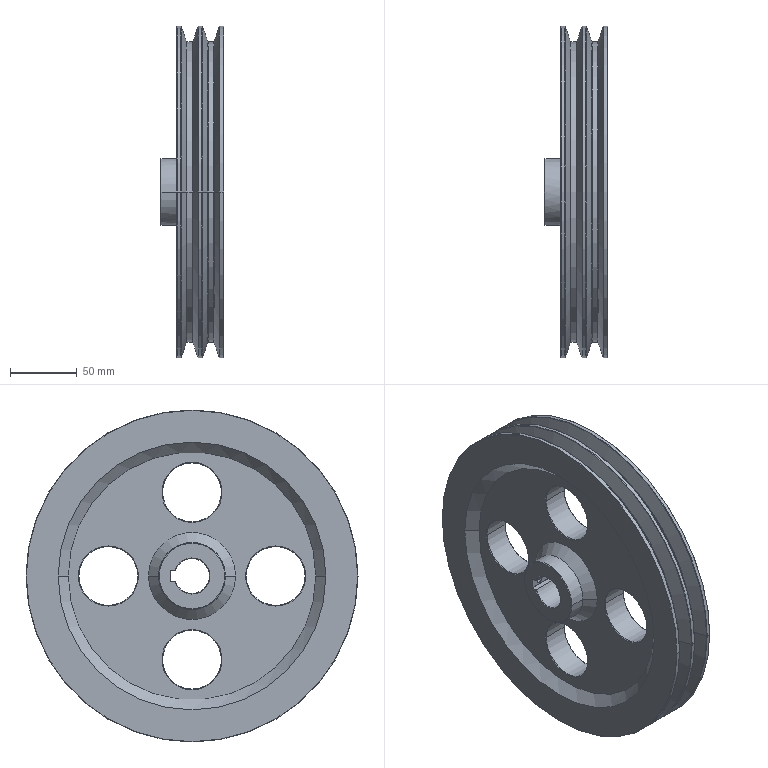Part | SolidWorks | features BaseBody 1 | 1 solid | 94 faces | box 47.331 x 248 x 248 mm | volume 1015220 mm3 | cone 52 | cylinder 25 | plane 9 | spline 8 | commonest cylinder face diameters 44 x8 248 x6 224.6 x4 0.32 x2 4.917 x2 50 x2